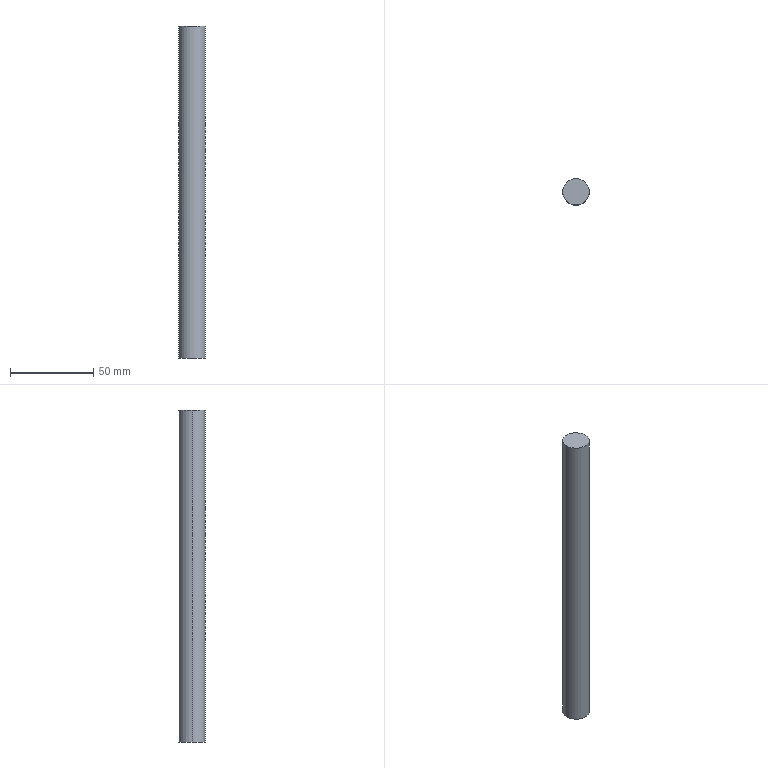Part | SolidWorks | features Extrusion 1 | 1 solid | 4 faces | box 16 x 16 x 200 mm | volume 40212 mm3 | cylinder 2 | plane 2 | commonest cylinder face diameters 16 x2
STEP:
#1=CARTESIAN_POINT('',(8.,0.,200.));
#2=VERTEX_POINT('',#1);
#3=CARTESIAN_POINT('',(-8.,0.,200.));
#4=VERTEX_POINT('',#3);
#5=CARTESIAN_POINT('',(0.,0.,200.));
#6=DIRECTION('',(0.,0.,1.));
#7=DIRECTION('',(1.,0.,0.));
#8=AXIS2_PLACEMENT_3D('',#5,#6,#7);
#9=CIRCLE('',#8,8.);
#10=EDGE_CURVE('',#2,#4,#9,.T.);
#11=ORIENTED_EDGE('',*,*,#10,.F.);
#12=CARTESIAN_POINT('',(8.,0.,0.));
#13=VERTEX_POINT('',#12);
#14=CARTESIAN_POINT('',(8.,0.,200.));
#15=DIRECTION('',(0.,0.,-1.));
#16=VECTOR('',#15,1000.);
#17=LINE('',#14,#16);
#18=EDGE_CURVE('',#2,#13,#17,.T.);
#19=ORIENTED_EDGE('',*,*,#18,.T.);
#20=CARTESIAN_POINT('',(-8.,0.,0.));
#21=VERTEX_POINT('',#20);
#22=CARTESIAN_POINT('',(0.,0.,0.));
#23=DIRECTION('',(0.,0.,1.));
#24=DIRECTION('',(1.,0.,0.));
#25=AXIS2_PLACEMENT_3D('',#22,#23,#24);
#26=CIRCLE('',#25,8.);
#27=EDGE_CURVE('',#13,#21,#26,.T.);
#28=ORIENTED_EDGE('',*,*,#27,.T.);
#29=CARTESIAN_POINT('',(-8.,0.,200.));
#30=DIRECTION('',(0.,0.,-1.));
#31=VECTOR('',#30,1000.);
#32=LINE('',#29,#31);
#33=EDGE_CURVE('',#4,#21,#32,.T.);
#34=ORIENTED_EDGE('',*,*,#33,.F.);
#35=EDGE_LOOP('',(#11,#19,#28,#34));
#36=FACE_OUTER_BOUND('',#35,.T.);
#37=CARTESIAN_POINT('',(0.,0.,200.));
#38=DIRECTION('',(0.,0.,-1.));
#39=DIRECTION('',(-1.,0.,0.));
#40=AXIS2_PLACEMENT_3D('',#37,#38,#39);
#41=CYLINDRICAL_SURFACE('',#40,8.);
#42=ADVANCED_FACE('',(#36),#41,.T.);
#43=ORIENTED_EDGE('',*,*,#18,.F.);
#44=CARTESIAN_POINT('',(0.,0.,200.));
#45=DIRECTION('',(0.,0.,1.));
#46=DIRECTION('',(1.,0.,0.));
#47=AXIS2_PLACEMENT_3D('',#44,#45,#46);
#48=CIRCLE('',#47,8.);
#49=EDGE_CURVE('',#4,#2,#48,.T.);
#50=ORIENTED_EDGE('',*,*,#49,.F.);
#51=ORIENTED_EDGE('',*,*,#33,.T.);
#52=CARTESIAN_POINT('',(0.,0.,0.));
#53=DIRECTION('',(0.,0.,1.));
#54=DIRECTION('',(1.,0.,0.));
#55=AXIS2_PLACEMENT_3D('',#52,#53,#54);
#56=CIRCLE('',#55,8.);
#57=EDGE_CURVE('',#21,#13,#56,.T.);
#58=ORIENTED_EDGE('',*,*,#57,.T.);
#59=EDGE_LOOP('',(#43,#50,#51,#58));
#60=FACE_OUTER_BOUND('',#59,.T.);
#61=CARTESIAN_POINT('',(0.,0.,200.));
#62=DIRECTION('',(0.,0.,-1.));
#63=DIRECTION('',(-1.,0.,0.));
#64=AXIS2_PLACEMENT_3D('',#61,#62,#63);
#65=CYLINDRICAL_SURFACE('',#64,8.);
#66=ADVANCED_FACE('',(#60),#65,.T.);
#67=ORIENTED_EDGE('',*,*,#49,.T.);
#68=ORIENTED_EDGE('',*,*,#10,.T.);
#69=EDGE_LOOP('',(#67,#68));
#70=FACE_OUTER_BOUND('',#69,.T.);
#71=CARTESIAN_POINT('',(0.,0.,200.));
#72=DIRECTION('',(0.,0.,1.));
#73=DIRECTION('',(1.,0.,0.));
#74=AXIS2_PLACEMENT_3D('',#71,#72,#73);
#75=PLANE('',#74);
#76=ADVANCED_FACE('',(#70),#75,.T.);
#77=ORIENTED_EDGE('',*,*,#57,.F.);
#78=ORIENTED_EDGE('',*,*,#27,.F.);
#79=EDGE_LOOP('',(#77,#78));
#80=FACE_OUTER_BOUND('',#79,.T.);
#81=CARTESIAN_POINT('',(0.,0.,0.));
#82=DIRECTION('',(0.,0.,1.));
#83=DIRECTION('',(1.,0.,0.));
#84=AXIS2_PLACEMENT_3D('',#81,#82,#83);
#85=PLANE('',#84);
#86=ADVANCED_FACE('',(#80),#85,.F.);
#87=CLOSED_SHELL('',(#42,#66,#76,#86));
#88=MANIFOLD_SOLID_BREP('',#87);
#89=CARTESIAN_POINT('',(0.,0.,0.));
#90=DIRECTION('',(0.,0.,1.));
#91=DIRECTION('',(1.,0.,0.));
#92=AXIS2_PLACEMENT_3D('',#89,#90,#91);
#93=(LENGTH_UNIT()NAMED_UNIT(*)SI_UNIT(.MILLI.,.METRE.));
#94=UNCERTAINTY_MEASURE_WITH_UNIT(LENGTH_MEASURE(0.00001),#93,'','');
#95=(NAMED_UNIT(*)PLANE_ANGLE_UNIT()SI_UNIT($,.RADIAN.));
#96=(NAMED_UNIT(*)SI_UNIT($,.STERADIAN.)SOLID_ANGLE_UNIT());
#97=(GEOMETRIC_REPRESENTATION_CONTEXT(3)GLOBAL_UNCERTAINTY_ASSIGNED_CONTEXT((#94))GLOBAL_UNIT_ASSIGNED_CONTEXT((#93,#95,#96))REPRESENTATION_CONTEXT('',''));
#98=ADVANCED_BREP_SHAPE_REPRESENTATION('',(#88,#92),#97);